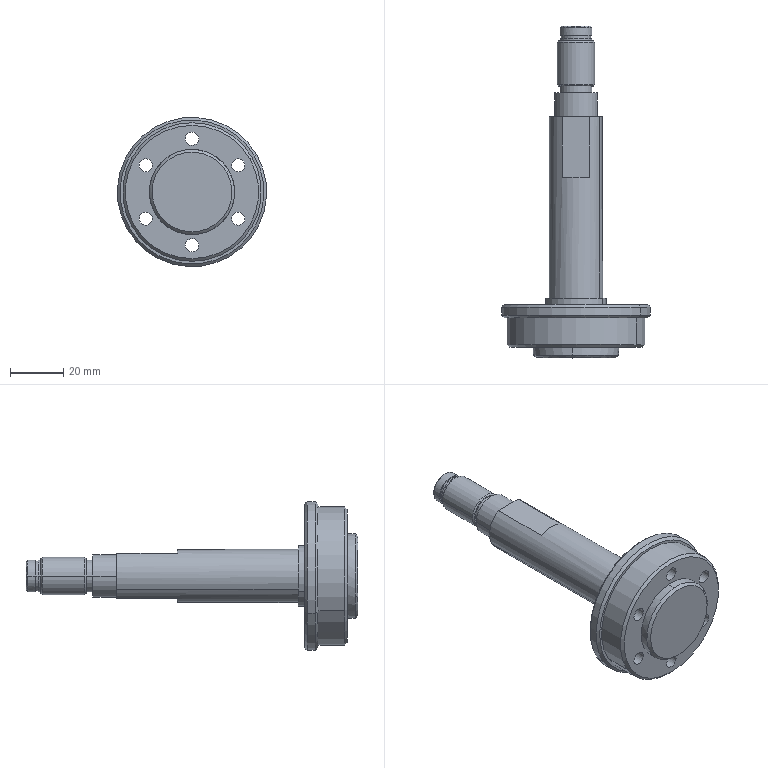Part | SolidWorks | features BaseBody 1 | 1 solid | 79 faces | box 56 x 124.5 x 56 mm | volume 63814 mm3 | cylinder 40 | plane 23 | cone 16 | commonest cylinder face diameters 5 x12 12 x6 2 x4 11 x2 14 x2 16 x2